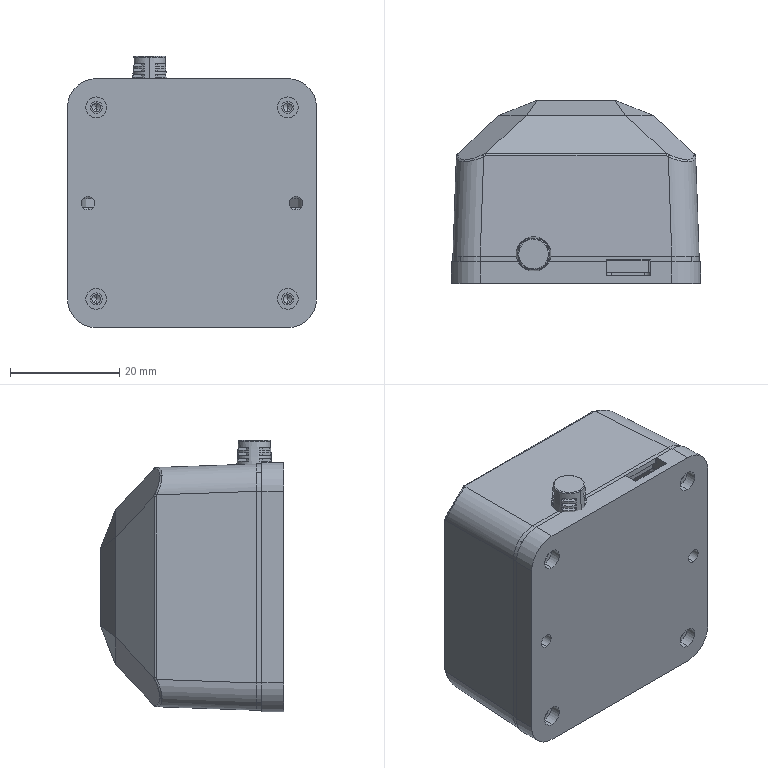Part | SolidWorks | features BaseBody 3, ICE 1 | 3 solids | 537 faces | box 45.5 x 33.5 x 49.567 mm | volume 18394 mm3 | plane 315 | cylinder 150 | spline 53 | cone 19 | commonest cylinder face diameters 2 x28 3.535 x14 1 x12 1.6 x12 3 x12 5 x12